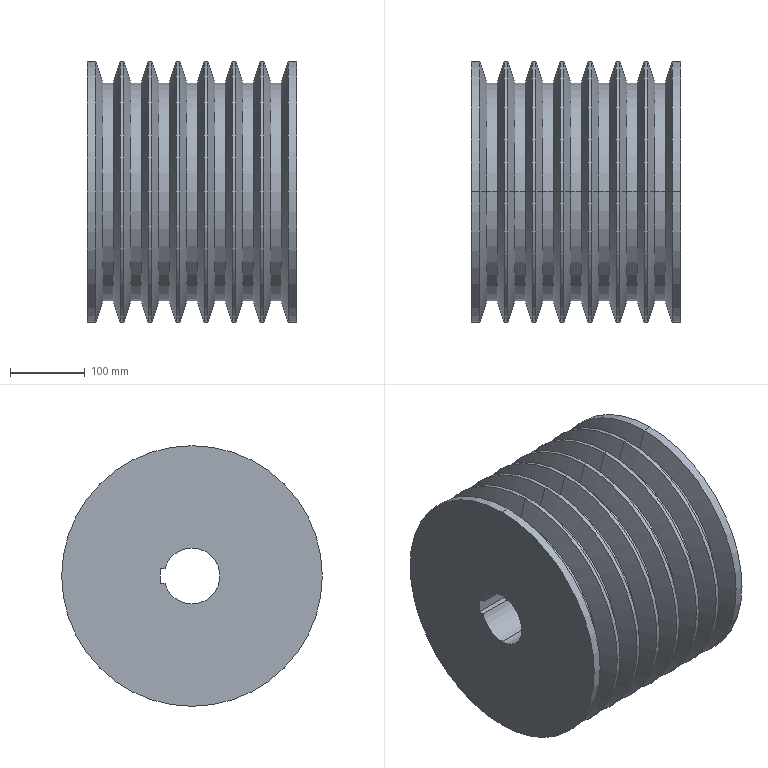Part | SolidWorks | features ICE 1, LPattern 1, RevCut 1, Revolution 1 | 1 solid | 69 faces | box 280 x 349 x 349 mm | volume 15090387 mm3 | cylinder 35 | cone 28 | plane 6 | commonest cylinder face diameters 349 x16 292 x14 75 x3 240 x2